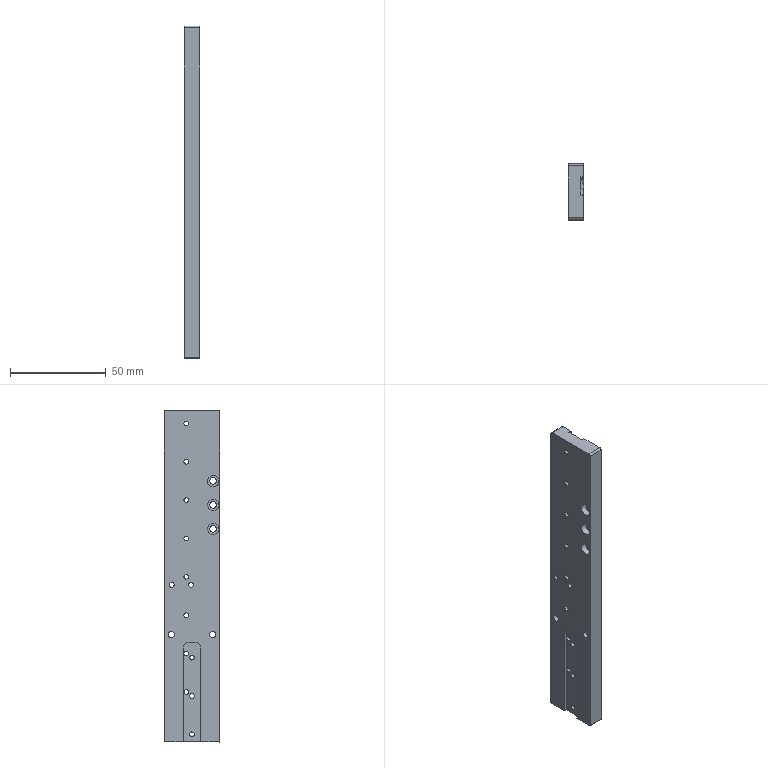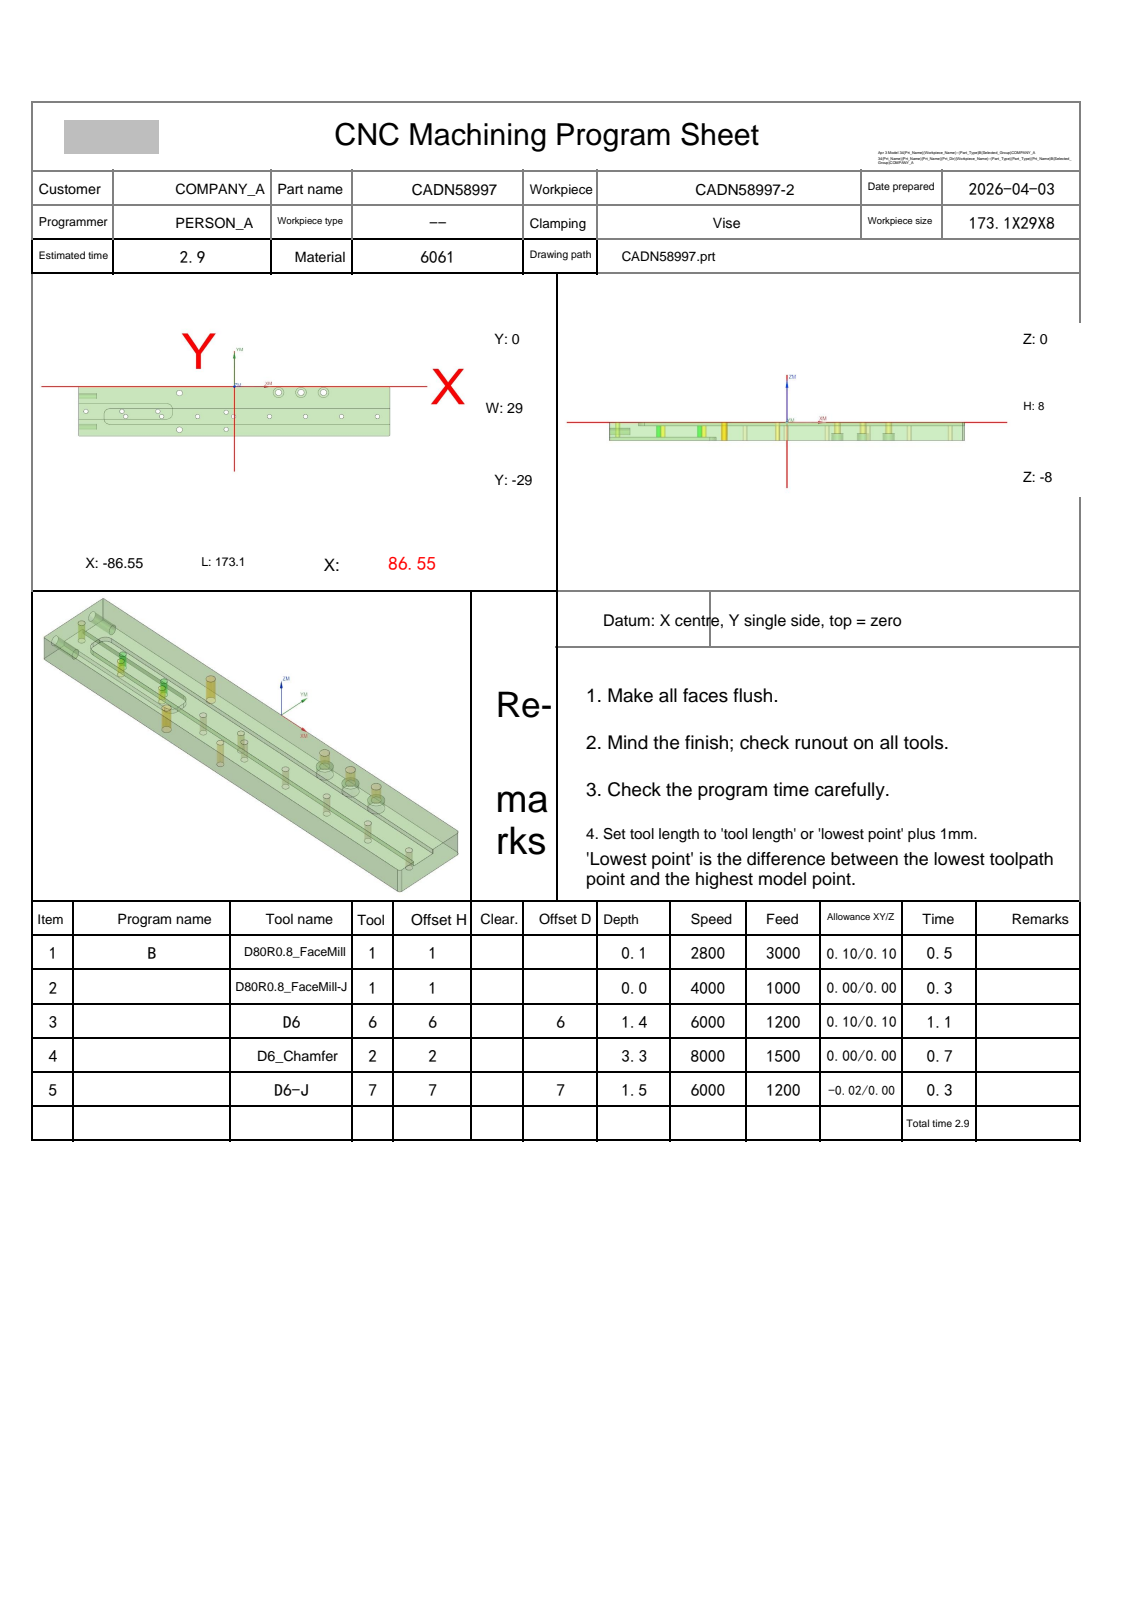NC program | NX | posted by the shop | part box 8 x 29 x 173.1 mm
Whole program:
%
O0001
(Machine time: 3.81 MIN)
(===Total Tool:4===)
(T1=D80R0.8 FaceMill D=80.  R=0.8  D-  H01 Z=-0.   )
(T6=D6      D=6.   R=0.   D6  H06 Z=-1.4  )
(T2=D6 Chamfer   D=6.   R=0.   D-  H02 Z=-3.25 )
(T7=D6-J    D=6.   R=0.   D7  H07 Z=-1.5  )
G80 G90 G17 G49 G40
G91 G28 Z0
M01
N1 T01 M06
(D80R0.8 FaceMill  D=80. R=0.8 H=01 ce=0.10 di=0.10)
G00 G90 G54 X138.647 Y-14.5 M03 S2800
G43 H01 Z20.
M08
Z3.525
G01 Z1.525 F3000.
X126.647
X-126.647
X-138.647
Z3.525
G00 X138.647
Z3.05
G01 Z1.05
X126.647
X-126.647
X-138.647
Z3.05
G00 X138.647
Z2.575
G01 Z.575
X126.647
X-126.647
X-138.647
Z2.575
G00 X138.647
Z2.1
G01 Z.1
X126.647
X-126.647
X-138.647
Z2.1
G00 Z20.
G91 G28 Z0.0
M05
M09
G91 G28 Z0.0
M01
N2 T01 M06
(D80R0.8 FaceMill-J  D=80. R=0.8 H=01 ce=0.00 di=0.00)
G00 G90 G54 X138.549 Y-14.5 M03 S4000
G43 H01 Z20.
M08
Z2.
G01 Z0.0 F1000.
X126.549
X-126.549
X-138.549
Z2.
G00 Z20.
G91 G28 Z0.0
M05
M09
G91 G28 Z0.0
M01
N3 T06 M06
(D6  D=6. R=0. H=06 ce=0.10 di=0.10)
G00 G90 G54 X90.746 Y-13.829 M03 S6000
G43 H06 Z20.
M08
Z.15
G01 Z-.35 F1200.
G41 D06
X90.65 Y-13.8
G03 X90.357 Y-13.756 I-.293 J-.956
X89.65 Y-14.049 I0.0 J-1.
G01 X87.634 Y-16.065
X-69.385
Y-18.935
X87.634
X89.65 Y-20.951
G03 X90.357 Y-21.244 I.707 J.707
X90.65 Y-21.2 I0.0 J1.
G01 G40 X90.746 Y-21.171
Z.15
G00 Z20.
Y-13.829
Z-.2
G01 Z-.7
G41 D06
X90.65 Y-13.8
G03 X90.357 Y-13.756 I-.293 J-.956
X89.65 Y-14.049 I0.0 J-1.
G01 X87.634 Y-16.065
X-69.385
Y-18.935
X87.634
X89.65 Y-20.951
G03 X90.357 Y-21.244 I.707 J.707
X90.65 Y-21.2 I0.0 J1.
G01 G40 X90.746 Y-21.171
Z-.2
G00 Z20.
Y-13.829
Z-.55
G01 Z-1.05
G41 D06
X90.65 Y-13.8
G03 X90.357 Y-13.756 I-.293 J-.956
X89.65 Y-14.049 I0.0 J-1.
G01 X87.634 Y-16.065
X-69.385
Y-18.935
X87.634
X89.65 Y-20.951
G03 X90.357 Y-21.244 I.707 J.707
X90.65 Y-21.2 I0.0 J1.
G01 G40 X90.746 Y-21.171
Z-.55
G00 Z20.
Y-13.829
Z-.9
G01 Z-1.4
G41 D06
X90.65 Y-13.8
G03 X90.357 Y-13.756 I-.293 J-.956
X89.65 Y-14.049 I0.0 J-1.
G01 X87.634 Y-16.065
X-69.385
Y-18.935
X87.634
X89.65 Y-20.951
G03 X90.357 Y-21.244 I.707 J.707
X90.65 Y-21.2 I0.0 J1.
G01 G40 X90.746 Y-21.171
Z-.9
G00 Z20.
G91 G28 Z0.0
M05
M09
G91 G28 Z0.0
M01
N4 T02 M06
(D6 Chamfer  D=6. R=0. H=02 ce=0.00 di=0.10)
G00 G90 G54 X-82.55 Y-14.5 M03 S8000
G43 H02 Z20.
M08
G98 G81 X-82.55 Y-14.5 Z-1.75 R3. F1000.
X-60.45 Y-17.5 Z-3.25 R1.5
X-40.45
X-20.45
X-4.574 Y-25.05 Z-1.75 R3.
X-.45 Y-17.5 Z-3.25 R1.5
X19.55
X39.55
X59.55
X79.55
G80
G00 Z20.
G00 G90 X-30.55 Y-3.75 M03 S8000
Z20.
G98 G81 X-30.55 Y-3.75 Z-2.2 R3. F1000.
Y-25.25
G80
G00 Z20.
G00 G90 X24.55 Y-3.455 M03 S8000
Z20.
G98 G81 X24.55 Y-3.455 Z-2.05 R3. F1000.
X37.05
X49.55
G80
G00 Z20.
G00 G90 X-.786 Y1.227 M03 S6500
Z20.
Z.172
G01 Z-1.199 F1500.
G03 X-.5 Y1.027 I1.286 J1.532
G01 X-.454 Y.997
X-.4 Y1.
X85.55
G02 X87.55 Y-1. I0.0 J-2.
G01 Y-12.765
X87.516 Y-13.024
X87.416 Y-13.265
X87.257 Y-13.472
X87.057 Y-13.672
X86.85 Y-13.831
X86.609 Y-13.931
X86.35 Y-13.965
X-69.45
G03 X-71.485 Y-16. I0.0 J-2.035
G01 Y-19.
G03 X-69.45 Y-21.035 I2.035 J0.0
G01 X86.35
X86.609 Y-21.069
X86.85 Y-21.169
X87.057 Y-21.328
X87.257 Y-21.528
X87.416 Y-21.735
X87.516 Y-21.976
X87.55 Y-22.235
Y-28.
G02 X85.55 Y-30. I-2. J0.0
G01 X-86.35
X-86.609 Y-29.966
X-86.85 Y-29.866
X-87.057 Y-29.707
X-87.257 Y-29.507
X-87.416 Y-29.3
X-87.516 Y-29.059
X-87.55 Y-28.8
Y-.2
X-87.516 Y.059
X-87.416 Y.3
X-87.257 Y.507
X-87.057 Y.707
X-86.85 Y.866
X-86.609 Y.966
X-86.35 Y1.
X-.4
X-.346 Y.997
X-.3 Y1.027
G03 X-.014 Y1.227 I-1. J1.732
G01 Z.172
G00 Z10.
X-31.044 Y-24.831
Z.405
G01 Z-1.199
G03 X-31.191 Y-25.147 I1.732 J-1.
G01 X-31.212 Y-25.197
X-31.2 Y-25.25
G03 X-30.55 Y-25.9 I.65 J0.0
X-29.9 Y-25.25 I0.0 J.65
X-30.55 Y-24.6 I-.65 J0.0
X-31.2 Y-25.25 I0.0 J-.65
G01 X-31.212 Y-25.303
X-31.191 Y-25.353
G03 X-31.044 Y-25.669 I1.879 J.684
G01 Z.405
G00 Z10.
Y-3.331
Z.405
G01 Z-1.199
G03 X-31.191 Y-3.647 I1.732 J-1.
G01 X-31.212 Y-3.697
X-31.2 Y-3.75
G03 X-30.55 Y-4.4 I.65 J0.0
X-29.9 Y-3.75 I0.0 J.65
X-30.55 Y-3.1 I-.65 J0.0
X-31.2 Y-3.75 I0.0 J-.65
G01 X-31.212 Y-3.803
X-31.191 Y-3.853
G03 X-31.044 Y-4.169 I1.879 J.684
G01 Z.405
G00 Z10.
X23.974 Y-3.043
Z.363
G01 Z-1.199
G03 X23.814 Y-3.352 I1.687 J-1.075
G01 X23.79 Y-3.401
X23.8 Y-3.455
G03 X24.55 Y-4.205 I.75 J0.0
X25.3 Y-3.455 I0.0 J.75
X24.55 Y-2.705 I-.75 J0.0
X23.826 Y-3.261 I0.0 J-.75
G01 X23.8 Y-3.455
X23.79 Y-3.509
X23.814 Y-3.558
G03 X23.974 Y-3.867 I1.848 J.765
G01 Z.363
G00 Z10.
X36.474 Y-3.043
Z.363
G01 Z-1.199
G03 X36.314 Y-3.352 I1.687 J-1.075
G01 X36.29 Y-3.401
X36.3 Y-3.455
G03 X37.05 Y-4.205 I.75 J0.0
X37.8 Y-3.455 I0.0 J.75
X37.05 Y-2.705 I-.75 J0.0
X36.326 Y-3.261 I0.0 J-.75
G01 X36.3 Y-3.455
X36.29 Y-3.509
X36.314 Y-3.558
G03 X36.474 Y-3.867 I1.848 J.765
G01 Z.363
G00 Z10.
X48.974 Y-3.043
Z.363
G01 Z-1.199
G03 X48.814 Y-3.352 I1.687 J-1.075
G01 X48.79 Y-3.401
X48.8 Y-3.455
G03 X49.55 Y-4.205 I.75 J0.0
X50.3 Y-3.455 I0.0 J.75
X49.55 Y-2.705 I-.75 J0.0
X48.826 Y-3.261 I0.0 J-.75
G01 X48.8 Y-3.455
X48.79 Y-3.509
X48.814 Y-3.558
G03 X48.974 Y-3.867 I1.848 J.765
G01 Z.363
G00 Z10.
X87.55 Y-15.354
Z1.301
G01 Z-2.699
Y-19.646
Z1.301
G00 Z20.
G91 G28 Z0.0
M05
M09
G91 G28 Z0.0
M01
N5 T07 M06
(D6-J  D=6. R=0. H=07 ce=-0.02 di=0.00)
G00 G90 G54 X90.63 Y-10.927 M03 S6000
G43 H07 Z20.
M08
Z-1.
G01 Z-1.5 F1200.
G41 D07
X90.53
G03 X89.53 Y-11.927 I0.0 J-1.
G01 Y-13.999
X87.584 Y-15.945
X-69.45
X-69.483 Y-15.944
X-69.506 Y-15.968
X-69.505 Y-16.
Y-19.
X-69.506 Y-19.033
X-69.483 Y-19.056
X-69.45 Y-19.055
X87.584
X89.53 Y-21.001
Y-23.073
G03 X90.53 Y-24.073 I1. J0.0
G01 G40 X90.63
Z-1.
G00 Z20.
M05
M09
G91 G28 Z0.0
G91 G28 Y0.0
M30
%